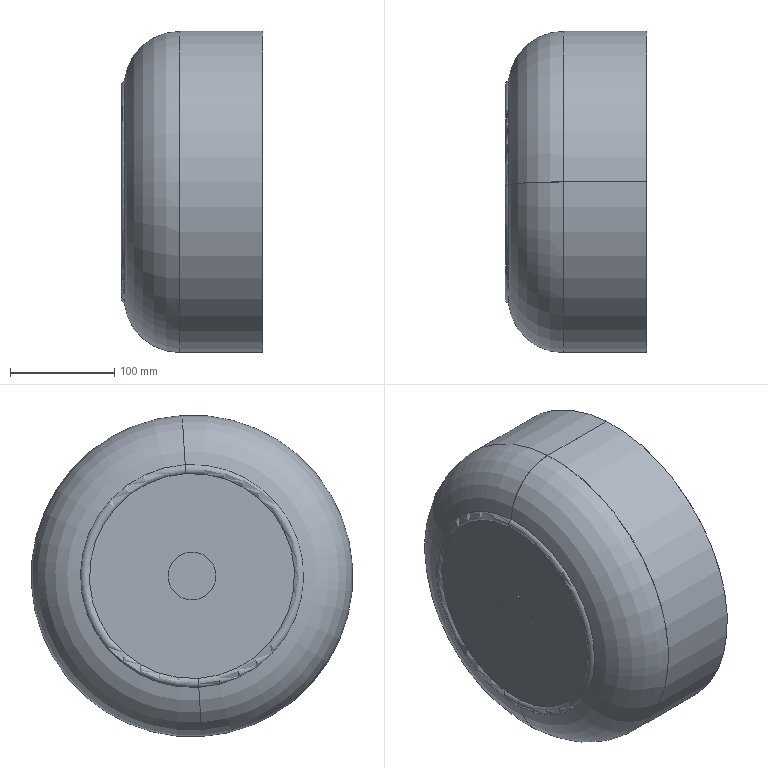Part | STEP file | Input 100 | 1 solid | 21 faces | box 136 x 309 x 309 mm | volume 181254 mm3 | cylinder 8 | torus 8 | plane 5 | commonest cylinder face diameters 44 x2 46 x2 307 x2 309 x2
STEP:
#1=CARTESIAN_POINT('',(0.,0.,0.));
#2=DIRECTION('',(0.,0.,1.));
#3=DIRECTION('',(1.,0.,0.));
#4=AXIS2_PLACEMENT_3D('',#1,#2,#3);
#5=CARTESIAN_POINT('',(3206.,663.657,-22.365));
#6=VERTEX_POINT('',#5);
#7=CARTESIAN_POINT('',(3207.,663.657,-22.365));
#8=VERTEX_POINT('',#7);
#9=CARTESIAN_POINT('',(3300.688,663.657,-22.365));
#10=DIRECTION('',(1.,0.,0.));
#11=VECTOR('',#10,1.);
#12=LINE('',#9,#11);
#13=CARTESIAN_POINT('',(3300.688,665.,-0.4063));
#14=DIRECTION('',(1.,0.,0.));
#15=DIRECTION('',(0.,-0.06105,-0.9981));
#16=AXIS2_PLACEMENT_3D('',#13,#14,#15);
#17=CYLINDRICAL_SURFACE('',#16,22.);
#18=CARTESIAN_POINT('',(6.283,0.));
#19=DIRECTION('',(0.,1.));
#20=VECTOR('',#19,1.);
#21=LINE('',#18,#20);
#22=(GEOMETRIC_REPRESENTATION_CONTEXT(2)PARAMETRIC_REPRESENTATION_CONTEXT()REPRESENTATION_CONTEXT('',''));
#23=DEFINITIONAL_REPRESENTATION('',(#21),#22);
#24=PCURVE('',#17,#23);
#25=CARTESIAN_POINT('',(3300.688,665.,-0.4063));
#26=DIRECTION('',(1.,0.,0.));
#27=DIRECTION('',(0.,-0.06105,-0.9981));
#28=AXIS2_PLACEMENT_3D('',#25,#26,#27);
#29=CYLINDRICAL_SURFACE('',#28,22.);
#30=CARTESIAN_POINT('',(0.,0.));
#31=DIRECTION('',(0.,1.));
#32=VECTOR('',#31,1.);
#33=LINE('',#30,#32);
#34=(GEOMETRIC_REPRESENTATION_CONTEXT(2)PARAMETRIC_REPRESENTATION_CONTEXT()REPRESENTATION_CONTEXT('',''));
#35=DEFINITIONAL_REPRESENTATION('',(#33),#34);
#36=PCURVE('',#29,#35);
#37=SURFACE_CURVE('',#12,(#24,#36),.PCURVE_S1.);
#38=EDGE_CURVE('',#6,#8,#37,.T.);
#39=ORIENTED_EDGE('',*,*,#38,.T.);
#40=CARTESIAN_POINT('',(3207.,666.343,21.553));
#41=VERTEX_POINT('',#40);
#42=CARTESIAN_POINT('',(3207.,665.,-0.4063));
#43=DIRECTION('',(1.,0.,0.));
#44=DIRECTION('',(0.,-0.06105,-0.9981));
#45=AXIS2_PLACEMENT_3D('',#42,#43,#44);
#46=CIRCLE('',#45,22.);
#47=CARTESIAN_POINT('',(0.,-93.688));
#48=DIRECTION('',(1.,0.));
#49=VECTOR('',#48,1.);
#50=LINE('',#47,#49);
#51=(GEOMETRIC_REPRESENTATION_CONTEXT(2)PARAMETRIC_REPRESENTATION_CONTEXT()REPRESENTATION_CONTEXT('',''));
#52=DEFINITIONAL_REPRESENTATION('',(#50),#51);
#53=PCURVE('',#17,#52);
#54=CARTESIAN_POINT('',(3207.,763.851,-6.452));
#55=DIRECTION('',(-1.,0.,0.));
#56=DIRECTION('',(0.,0.06105,0.9981));
#57=AXIS2_PLACEMENT_3D('',#54,#55,#56);
#58=PLANE('',#57);
#59=CARTESIAN_POINT('',(-22.,-99.036));
#60=CARTESIAN_POINT('',(-22.,-60.931));
#61=CARTESIAN_POINT('',(11.,-79.983));
#62=CARTESIAN_POINT('',(44.,-99.036));
#63=CARTESIAN_POINT('',(11.,-118.088));
#64=CARTESIAN_POINT('',(-22.,-137.141));
#65=CARTESIAN_POINT('',(-22.,-99.036));
#66=(BOUNDED_CURVE()B_SPLINE_CURVE(2,(#59,#60,#61,#62,#63,#64,#65),.UNSPECIFIED.,.T.,.F.)B_SPLINE_CURVE_WITH_KNOTS((1,2,2,2,2,1),(-2.094,0.,2.094,4.189,6.283,8.378),.UNSPECIFIED.)CURVE()GEOMETRIC_REPRESENTATION_ITEM()RATIONAL_B_SPLINE_CURVE((1.,0.5,1.,0.5,1.,0.5,1.))REPRESENTATION_ITEM(''));
#67=(GEOMETRIC_REPRESENTATION_CONTEXT(2)PARAMETRIC_REPRESENTATION_CONTEXT()REPRESENTATION_CONTEXT('',''));
#68=DEFINITIONAL_REPRESENTATION('',(#66),#67);
#69=PCURVE('',#58,#68);
#70=SURFACE_CURVE('',#46,(#53,#69),.PCURVE_S1.);
#71=EDGE_CURVE('',#41,#8,#70,.T.);
#72=ORIENTED_EDGE('',*,*,#71,.F.);
#73=CARTESIAN_POINT('',(3206.,666.343,21.553));
#74=VERTEX_POINT('',#73);
#75=CARTESIAN_POINT('',(3300.688,666.343,21.553));
#76=DIRECTION('',(1.,0.,0.));
#77=VECTOR('',#76,1.);
#78=LINE('',#75,#77);
#79=CARTESIAN_POINT('',(3.142,0.));
#80=DIRECTION('',(0.,1.));
#81=VECTOR('',#80,1.);
#82=LINE('',#79,#81);
#83=(GEOMETRIC_REPRESENTATION_CONTEXT(2)PARAMETRIC_REPRESENTATION_CONTEXT()REPRESENTATION_CONTEXT('',''));
#84=DEFINITIONAL_REPRESENTATION('',(#82),#83);
#85=PCURVE('',#17,#84);
#86=CARTESIAN_POINT('',(3.142,0.));
#87=DIRECTION('',(0.,1.));
#88=VECTOR('',#87,1.);
#89=LINE('',#86,#88);
#90=(GEOMETRIC_REPRESENTATION_CONTEXT(2)PARAMETRIC_REPRESENTATION_CONTEXT()REPRESENTATION_CONTEXT('',''));
#91=DEFINITIONAL_REPRESENTATION('',(#89),#90);
#92=PCURVE('',#29,#91);
#93=SURFACE_CURVE('',#78,(#85,#92),.PCURVE_S1.);
#94=EDGE_CURVE('',#74,#41,#93,.T.);
#95=ORIENTED_EDGE('',*,*,#94,.F.);
#96=CARTESIAN_POINT('',(3206.,665.,-0.4063));
#97=DIRECTION('',(1.,0.,0.));
#98=DIRECTION('',(0.,-0.06105,-0.9981));
#99=AXIS2_PLACEMENT_3D('',#96,#97,#98);
#100=CIRCLE('',#99,22.);
#101=CARTESIAN_POINT('',(0.,-94.688));
#102=DIRECTION('',(1.,0.));
#103=VECTOR('',#102,1.);
#104=LINE('',#101,#103);
#105=(GEOMETRIC_REPRESENTATION_CONTEXT(2)PARAMETRIC_REPRESENTATION_CONTEXT()REPRESENTATION_CONTEXT('',''));
#106=DEFINITIONAL_REPRESENTATION('',(#104),#105);
#107=PCURVE('',#17,#106);
#108=CARTESIAN_POINT('',(3206.,686.959,-1.749));
#109=DIRECTION('',(-1.,0.,0.));
#110=DIRECTION('',(0.,0.06105,0.9981));
#111=AXIS2_PLACEMENT_3D('',#108,#109,#110);
#112=PLANE('',#111);
#113=CARTESIAN_POINT('',(-22.,-22.));
#114=CARTESIAN_POINT('',(-22.,16.105));
#115=CARTESIAN_POINT('',(11.,-2.947));
#116=CARTESIAN_POINT('',(44.,-22.));
#117=CARTESIAN_POINT('',(11.,-41.053));
#118=CARTESIAN_POINT('',(-22.,-60.105));
#119=CARTESIAN_POINT('',(-22.,-22.));
#120=(BOUNDED_CURVE()B_SPLINE_CURVE(2,(#113,#114,#115,#116,#117,#118,#119),.UNSPECIFIED.,.T.,.F.)B_SPLINE_CURVE_WITH_KNOTS((1,2,2,2,2,1),(-2.094,0.,2.094,4.189,6.283,8.378),.UNSPECIFIED.)CURVE()GEOMETRIC_REPRESENTATION_ITEM()RATIONAL_B_SPLINE_CURVE((1.,0.5,1.,0.5,1.,0.5,1.))REPRESENTATION_ITEM(''));
#121=(GEOMETRIC_REPRESENTATION_CONTEXT(2)PARAMETRIC_REPRESENTATION_CONTEXT()REPRESENTATION_CONTEXT('',''));
#122=DEFINITIONAL_REPRESENTATION('',(#120),#121);
#123=PCURVE('',#112,#122);
#124=SURFACE_CURVE('',#100,(#107,#123),.PCURVE_S1.);
#125=EDGE_CURVE('',#74,#6,#124,.T.);
#126=ORIENTED_EDGE('',*,*,#125,.T.);
#127=EDGE_LOOP('',(#39,#72,#95,#126));
#128=FACE_BOUND('',#127,.F.);
#129=ADVANCED_FACE('',(#128),#17,.F.);
#130=CARTESIAN_POINT('',(3260.,655.629,-153.62));
#131=VERTEX_POINT('',#130);
#132=CARTESIAN_POINT('',(3340.,655.629,-153.62));
#133=VERTEX_POINT('',#132);
#134=CARTESIAN_POINT('',(3300.688,655.629,-153.62));
#135=DIRECTION('',(1.,0.,0.));
#136=VECTOR('',#135,1.);
#137=LINE('',#134,#136);
#138=CARTESIAN_POINT('',(3300.688,665.,-0.4063));
#139=DIRECTION('',(1.,0.,0.));
#140=DIRECTION('',(0.,-0.06105,-0.9981));
#141=AXIS2_PLACEMENT_3D('',#138,#139,#140);
#142=CYLINDRICAL_SURFACE('',#141,153.5);
#143=CARTESIAN_POINT('',(6.283,0.));
#144=DIRECTION('',(0.,1.));
#145=VECTOR('',#144,1.);
#146=LINE('',#143,#145);
#147=(GEOMETRIC_REPRESENTATION_CONTEXT(2)PARAMETRIC_REPRESENTATION_CONTEXT()REPRESENTATION_CONTEXT('',''));
#148=DEFINITIONAL_REPRESENTATION('',(#146),#147);
#149=PCURVE('',#142,#148);
#150=CARTESIAN_POINT('',(3300.688,665.,-0.4063));
#151=DIRECTION('',(1.,0.,0.));
#152=DIRECTION('',(0.,-0.06105,-0.9981));
#153=AXIS2_PLACEMENT_3D('',#150,#151,#152);
#154=CYLINDRICAL_SURFACE('',#153,153.5);
#155=CARTESIAN_POINT('',(0.,0.));
#156=DIRECTION('',(0.,1.));
#157=VECTOR('',#156,1.);
#158=LINE('',#155,#157);
#159=(GEOMETRIC_REPRESENTATION_CONTEXT(2)PARAMETRIC_REPRESENTATION_CONTEXT()REPRESENTATION_CONTEXT('',''));
#160=DEFINITIONAL_REPRESENTATION('',(#158),#159);
#161=PCURVE('',#154,#160);
#162=SURFACE_CURVE('',#137,(#149,#161),.PCURVE_S1.);
#163=EDGE_CURVE('',#131,#133,#162,.T.);
#164=ORIENTED_EDGE('',*,*,#163,.T.);
#165=CARTESIAN_POINT('',(3340.,674.371,152.807));
#166=VERTEX_POINT('',#165);
#167=CARTESIAN_POINT('',(3340.,665.,-0.4063));
#168=DIRECTION('',(1.,0.,0.));
#169=DIRECTION('',(0.,-0.06105,-0.9981));
#170=AXIS2_PLACEMENT_3D('',#167,#168,#169);
#171=CIRCLE('',#170,153.5);
#172=CARTESIAN_POINT('',(0.,39.312));
#173=DIRECTION('',(1.,0.));
#174=VECTOR('',#173,1.);
#175=LINE('',#172,#174);
#176=(GEOMETRIC_REPRESENTATION_CONTEXT(2)PARAMETRIC_REPRESENTATION_CONTEXT()REPRESENTATION_CONTEXT('',''));
#177=DEFINITIONAL_REPRESENTATION('',(#175),#176);
#178=PCURVE('',#142,#177);
#179=CARTESIAN_POINT('',(3340.,665.,-0.4063));
#180=DIRECTION('',(-1.,0.,0.));
#181=DIRECTION('',(0.,0.06105,0.9981));
#182=AXIS2_PLACEMENT_3D('',#179,#180,#181);
#183=PLANE('',#182);
#184=CARTESIAN_POINT('',(-153.5,0.));
#185=CARTESIAN_POINT('',(-153.5,265.87));
#186=CARTESIAN_POINT('',(76.75,132.935));
#187=CARTESIAN_POINT('',(307.,0.));
#188=CARTESIAN_POINT('',(76.75,-132.935));
#189=CARTESIAN_POINT('',(-153.5,-265.87));
#190=CARTESIAN_POINT('',(-153.5,0.));
#191=(BOUNDED_CURVE()B_SPLINE_CURVE(2,(#184,#185,#186,#187,#188,#189,#190),.UNSPECIFIED.,.T.,.F.)B_SPLINE_CURVE_WITH_KNOTS((1,2,2,2,2,1),(-2.094,0.,2.094,4.189,6.283,8.378),.UNSPECIFIED.)CURVE()GEOMETRIC_REPRESENTATION_ITEM()RATIONAL_B_SPLINE_CURVE((1.,0.5,1.,0.5,1.,0.5,1.))REPRESENTATION_ITEM(''));
#192=(GEOMETRIC_REPRESENTATION_CONTEXT(2)PARAMETRIC_REPRESENTATION_CONTEXT()REPRESENTATION_CONTEXT('',''));
#193=DEFINITIONAL_REPRESENTATION('',(#191),#192);
#194=PCURVE('',#183,#193);
#195=SURFACE_CURVE('',#171,(#178,#194),.PCURVE_S1.);
#196=EDGE_CURVE('',#166,#133,#195,.T.);
#197=ORIENTED_EDGE('',*,*,#196,.F.);
#198=CARTESIAN_POINT('',(3260.,674.371,152.807));
#199=VERTEX_POINT('',#198);
#200=CARTESIAN_POINT('',(3300.688,674.371,152.807));
#201=DIRECTION('',(1.,0.,0.));
#202=VECTOR('',#201,1.);
#203=LINE('',#200,#202);
#204=CARTESIAN_POINT('',(3.142,0.));
#205=DIRECTION('',(0.,1.));
#206=VECTOR('',#205,1.);
#207=LINE('',#204,#206);
#208=(GEOMETRIC_REPRESENTATION_CONTEXT(2)PARAMETRIC_REPRESENTATION_CONTEXT()REPRESENTATION_CONTEXT('',''));
#209=DEFINITIONAL_REPRESENTATION('',(#207),#208);
#210=PCURVE('',#142,#209);
#211=CARTESIAN_POINT('',(3.142,0.));
#212=DIRECTION('',(0.,1.));
#213=VECTOR('',#212,1.);
#214=LINE('',#211,#213);
#215=(GEOMETRIC_REPRESENTATION_CONTEXT(2)PARAMETRIC_REPRESENTATION_CONTEXT()REPRESENTATION_CONTEXT('',''));
#216=DEFINITIONAL_REPRESENTATION('',(#214),#215);
#217=PCURVE('',#154,#216);
#218=SURFACE_CURVE('',#203,(#210,#217),.PCURVE_S1.);
#219=EDGE_CURVE('',#199,#166,#218,.T.);
#220=ORIENTED_EDGE('',*,*,#219,.F.);
#221=CARTESIAN_POINT('',(3260.,665.,-0.4063));
#222=DIRECTION('',(1.,0.,0.));
#223=DIRECTION('',(0.,-0.06105,-0.9981));
#224=AXIS2_PLACEMENT_3D('',#221,#222,#223);
#225=CIRCLE('',#224,153.5);
#226=CARTESIAN_POINT('',(0.,-40.688));
#227=DIRECTION('',(1.,0.));
#228=VECTOR('',#227,1.);
#229=LINE('',#226,#228);
#230=(GEOMETRIC_REPRESENTATION_CONTEXT(2)PARAMETRIC_REPRESENTATION_CONTEXT()REPRESENTATION_CONTEXT('',''));
#231=DEFINITIONAL_REPRESENTATION('',(#229),#230);
#232=PCURVE('',#142,#231);
#233=CARTESIAN_POINT('',(3260.,665.,-0.4063));
#234=DIRECTION('',(1.,0.,0.));
#235=DIRECTION('',(0.,-0.06105,-0.9981));
#236=AXIS2_PLACEMENT_3D('',#233,#234,#235);
#237=TOROIDAL_SURFACE('',#236,101.248,52.252);
#238=CARTESIAN_POINT('',(0.,6.283));
#239=DIRECTION('',(1.,0.));
#240=VECTOR('',#239,1.);
#241=LINE('',#238,#240);
#242=(GEOMETRIC_REPRESENTATION_CONTEXT(2)PARAMETRIC_REPRESENTATION_CONTEXT()REPRESENTATION_CONTEXT('',''));
#243=DEFINITIONAL_REPRESENTATION('',(#241),#242);
#244=PCURVE('',#237,#243);
#245=SURFACE_CURVE('',#225,(#232,#244),.PCURVE_S1.);
#246=EDGE_CURVE('',#199,#131,#245,.T.);
#247=ORIENTED_EDGE('',*,*,#246,.T.);
#248=EDGE_LOOP('',(#164,#197,#220,#247));
#249=FACE_BOUND('',#248,.F.);
#250=ADVANCED_FACE('',(#249),#142,.F.);
#251=CARTESIAN_POINT('',(3207.,658.954,-99.257));
#252=VERTEX_POINT('',#251);
#253=CARTESIAN_POINT('',(3208.,658.506,-106.581));
#254=VERTEX_POINT('',#253);
#255=CARTESIAN_POINT('',(3209.,658.743,-102.715));
#256=DIRECTION('',(0.,-0.9981,0.06105));
#257=DIRECTION('',(0.,-0.06105,-0.9981));
#258=AXIS2_PLACEMENT_3D('',#255,#256,#257);
#259=CIRCLE('',#258,4.);
#260=CARTESIAN_POINT('',(3209.,665.,-0.4063));
#261=DIRECTION('',(1.,0.,0.));
#262=DIRECTION('',(0.,-0.06105,-0.9981));
#263=AXIS2_PLACEMENT_3D('',#260,#261,#262);
#264=TOROIDAL_SURFACE('',#263,102.5,4.);
#265=CARTESIAN_POINT('',(6.283,0.));
#266=DIRECTION('',(0.,1.));
#267=VECTOR('',#266,1.);
#268=LINE('',#265,#267);
#269=(GEOMETRIC_REPRESENTATION_CONTEXT(2)PARAMETRIC_REPRESENTATION_CONTEXT()REPRESENTATION_CONTEXT('',''));
#270=DEFINITIONAL_REPRESENTATION('',(#268),#269);
#271=PCURVE('',#264,#270);
#272=CARTESIAN_POINT('',(3209.,665.,-0.4063));
#273=DIRECTION('',(1.,0.,0.));
#274=DIRECTION('',(0.,-0.06105,-0.9981));
#275=AXIS2_PLACEMENT_3D('',#272,#273,#274);
#276=TOROIDAL_SURFACE('',#275,102.5,4.);
#277=CARTESIAN_POINT('',(0.,0.));
#278=DIRECTION('',(0.,1.));
#279=VECTOR('',#278,1.);
#280=LINE('',#277,#279);
#281=(GEOMETRIC_REPRESENTATION_CONTEXT(2)PARAMETRIC_REPRESENTATION_CONTEXT()REPRESENTATION_CONTEXT('',''));
#282=DEFINITIONAL_REPRESENTATION('',(#280),#281);
#283=PCURVE('',#276,#282);
#284=SURFACE_CURVE('',#259,(#271,#283),.PCURVE_S1.);
#285=EDGE_CURVE('',#252,#254,#284,.T.);
#286=ORIENTED_EDGE('',*,*,#285,.T.);
#287=CARTESIAN_POINT('',(3208.,671.494,105.768));
#288=VERTEX_POINT('',#287);
#289=CARTESIAN_POINT('',(3208.,665.,-0.4063));
#290=DIRECTION('',(1.,0.,0.));
#291=DIRECTION('',(0.,-0.06105,-0.9981));
#292=AXIS2_PLACEMENT_3D('',#289,#290,#291);
#293=CIRCLE('',#292,106.373);
#294=CARTESIAN_POINT('',(0.,6.031));
#295=DIRECTION('',(1.,0.));
#296=VECTOR('',#295,1.);
#297=LINE('',#294,#296);
#298=(GEOMETRIC_REPRESENTATION_CONTEXT(2)PARAMETRIC_REPRESENTATION_CONTEXT()REPRESENTATION_CONTEXT('',''));
#299=DEFINITIONAL_REPRESENTATION('',(#297),#298);
#300=PCURVE('',#264,#299);
#301=CARTESIAN_POINT('',(0.,4.811));
#302=DIRECTION('',(1.,0.));
#303=VECTOR('',#302,1.);
#304=LINE('',#301,#303);
#305=(GEOMETRIC_REPRESENTATION_CONTEXT(2)PARAMETRIC_REPRESENTATION_CONTEXT()REPRESENTATION_CONTEXT('',''));
#306=DEFINITIONAL_REPRESENTATION('',(#304),#305);
#307=PCURVE('',#237,#306);
#308=SURFACE_CURVE('',#293,(#300,#307),.PCURVE_S1.);
#309=EDGE_CURVE('',#288,#254,#308,.T.);
#310=ORIENTED_EDGE('',*,*,#309,.F.);
#311=CARTESIAN_POINT('',(3207.,671.046,98.445));
#312=VERTEX_POINT('',#311);
#313=CARTESIAN_POINT('',(3209.,671.257,101.902));
#314=DIRECTION('',(0.,0.9981,-0.06105));
#315=DIRECTION('',(0.,0.06105,0.9981));
#316=AXIS2_PLACEMENT_3D('',#313,#314,#315);
#317=CIRCLE('',#316,4.);
#318=CARTESIAN_POINT('',(3.142,0.));
#319=DIRECTION('',(0.,1.));
#320=VECTOR('',#319,1.);
#321=LINE('',#318,#320);
#322=(GEOMETRIC_REPRESENTATION_CONTEXT(2)PARAMETRIC_REPRESENTATION_CONTEXT()REPRESENTATION_CONTEXT('',''));
#323=DEFINITIONAL_REPRESENTATION('',(#321),#322);
#324=PCURVE('',#264,#323);
#325=CARTESIAN_POINT('',(3.142,0.));
#326=DIRECTION('',(0.,1.));
#327=VECTOR('',#326,1.);
#328=LINE('',#325,#327);
#329=(GEOMETRIC_REPRESENTATION_CONTEXT(2)PARAMETRIC_REPRESENTATION_CONTEXT()REPRESENTATION_CONTEXT('',''));
#330=DEFINITIONAL_REPRESENTATION('',(#328),#329);
#331=PCURVE('',#276,#330);
#332=SURFACE_CURVE('',#317,(#324,#331),.PCURVE_S1.);
#333=EDGE_CURVE('',#312,#288,#332,.T.);
#334=ORIENTED_EDGE('',*,*,#333,.F.);
#335=CARTESIAN_POINT('',(3207.,665.,-0.4063));
#336=DIRECTION('',(1.,0.,0.));
#337=DIRECTION('',(0.,-0.06105,-0.9981));
#338=AXIS2_PLACEMENT_3D('',#335,#336,#337);
#339=CIRCLE('',#338,99.036);
#340=CARTESIAN_POINT('',(0.,3.665));
#341=DIRECTION('',(1.,0.));
#342=VECTOR('',#341,1.);
#343=LINE('',#340,#342);
#344=(GEOMETRIC_REPRESENTATION_CONTEXT(2)PARAMETRIC_REPRESENTATION_CONTEXT()REPRESENTATION_CONTEXT('',''));
#345=DEFINITIONAL_REPRESENTATION('',(#343),#344);
#346=PCURVE('',#264,#345);
#347=CARTESIAN_POINT('',(-99.036,-99.036));
#348=CARTESIAN_POINT('',(-99.036,72.499));
#349=CARTESIAN_POINT('',(49.518,-13.268));
#350=CARTESIAN_POINT('',(198.072,-99.036));
#351=CARTESIAN_POINT('',(49.518,-184.804));
#352=CARTESIAN_POINT('',(-99.036,-270.571));
#353=CARTESIAN_POINT('',(-99.036,-99.036));
#354=(BOUNDED_CURVE()B_SPLINE_CURVE(2,(#347,#348,#349,#350,#351,#352,#353),.UNSPECIFIED.,.T.,.F.)B_SPLINE_CURVE_WITH_KNOTS((1,2,2,2,2,1),(-2.094,0.,2.094,4.189,6.283,8.378),.UNSPECIFIED.)CURVE()GEOMETRIC_REPRESENTATION_ITEM()RATIONAL_B_SPLINE_CURVE((1.,0.5,1.,0.5,1.,0.5,1.))REPRESENTATION_ITEM(''));
#355=(GEOMETRIC_REPRESENTATION_CONTEXT(2)PARAMETRIC_REPRESENTATION_CONTEXT()REPRESENTATION_CONTEXT('',''));
#356=DEFINITIONAL_REPRESENTATION('',(#354),#355);
#357=PCURVE('',#58,#356);
#358=SURFACE_CURVE('',#339,(#346,#357),.PCURVE_S1.);
#359=EDGE_CURVE('',#312,#252,#358,.T.);
#360=ORIENTED_EDGE('',*,*,#359,.T.);
#361=EDGE_LOOP('',(#286,#310,#334,#360));
#362=FACE_BOUND('',#361,.F.);
#363=ADVANCED_FACE('',(#362),#264,.F.);
#364=CARTESIAN_POINT('',(3260.,658.819,-101.466));
#365=DIRECTION('',(0.,-0.9981,0.06105));
#366=DIRECTION('',(0.,-0.06105,-0.9981));
#367=AXIS2_PLACEMENT_3D('',#364,#365,#366);
#368=CIRCLE('',#367,52.252);
#369=CARTESIAN_POINT('',(6.283,0.));
#370=DIRECTION('',(0.,1.));
#371=VECTOR('',#370,1.);
#372=LINE('',#369,#371);
#373=(GEOMETRIC_REPRESENTATION_CONTEXT(2)PARAMETRIC_REPRESENTATION_CONTEXT()REPRESENTATION_CONTEXT('',''));
#374=DEFINITIONAL_REPRESENTATION('',(#372),#373);
#375=PCURVE('',#237,#374);
#376=CARTESIAN_POINT('',(3260.,665.,-0.4063));
#377=DIRECTION('',(1.,0.,0.));
#378=DIRECTION('',(0.,-0.06105,-0.9981));
#379=AXIS2_PLACEMENT_3D('',#376,#377,#378);
#380=TOROIDAL_SURFACE('',#379,101.248,52.252);
#381=CARTESIAN_POINT('',(0.,0.));
#382=DIRECTION('',(0.,1.));
#383=VECTOR('',#382,1.);
#384=LINE('',#381,#383);
#385=(GEOMETRIC_REPRESENTATION_CONTEXT(2)PARAMETRIC_REPRESENTATION_CONTEXT()REPRESENTATION_CONTEXT('',''));
#386=DEFINITIONAL_REPRESENTATION('',(#384),#385);
#387=PCURVE('',#380,#386);
#388=SURFACE_CURVE('',#368,(#375,#387),.PCURVE_S1.);
#389=EDGE_CURVE('',#254,#131,#388,.T.);
#390=ORIENTED_EDGE('',*,*,#389,.T.);
#391=ORIENTED_EDGE('',*,*,#246,.F.);
#392=CARTESIAN_POINT('',(3260.,671.181,100.653));
#393=DIRECTION('',(0.,0.9981,-0.06105));
#394=DIRECTION('',(0.,0.06105,0.9981));
#395=AXIS2_PLACEMENT_3D('',#392,#393,#394);
#396=CIRCLE('',#395,52.252);
#397=CARTESIAN_POINT('',(3.142,0.));
#398=DIRECTION('',(0.,1.));
#399=VECTOR('',#398,1.);
#400=LINE('',#397,#399);
#401=(GEOMETRIC_REPRESENTATION_CONTEXT(2)PARAMETRIC_REPRESENTATION_CONTEXT()REPRESENTATION_CONTEXT('',''));
#402=DEFINITIONAL_REPRESENTATION('',(#400),#401);
#403=PCURVE('',#237,#402);
#404=CARTESIAN_POINT('',(3.142,0.));
#405=DIRECTION('',(0.,1.));
#406=VECTOR('',#405,1.);
#407=LINE('',#404,#406);
#408=(GEOMETRIC_REPRESENTATION_CONTEXT(2)PARAMETRIC_REPRESENTATION_CONTEXT()REPRESENTATION_CONTEXT('',''));
#409=DEFINITIONAL_REPRESENTATION('',(#407),#408);
#410=PCURVE('',#380,#409);
#411=SURFACE_CURVE('',#396,(#403,#410),.PCURVE_S1.);
#412=EDGE_CURVE('',#288,#199,#411,.T.);
#413=ORIENTED_EDGE('',*,*,#412,.F.);
#414=ORIENTED_EDGE('',*,*,#309,.T.);
#415=EDGE_LOOP('',(#390,#391,#413,#414));
#416=FACE_BOUND('',#415,.F.);
#417=ADVANCED_FACE('',(#416),#237,.F.);
#418=CARTESIAN_POINT('',(3205.,663.596,-23.363));
#419=VERTEX_POINT('',#418);
#420=CARTESIAN_POINT('',(3205.,666.404,22.551));
#421=VERTEX_POINT('',#420);
#422=CARTESIAN_POINT('',(3205.,665.,-0.4063));
#423=DIRECTION('',(1.,0.,0.));
#424=DIRECTION('',(0.,0.06105,0.9981));
#425=AXIS2_PLACEMENT_3D('',#422,#423,#424);
#426=CIRCLE('',#425,23.);
#427=CARTESIAN_POINT('',(3300.688,665.,-0.4063));
#428=DIRECTION('',(1.,0.,0.));
#429=DIRECTION('',(0.,-0.06105,-0.9981));
#430=AXIS2_PLACEMENT_3D('',#427,#428,#429);
#431=CYLINDRICAL_SURFACE('',#430,23.);
#432=CARTESIAN_POINT('',(-3.142,-95.688));
#433=DIRECTION('',(1.,0.));
#434=VECTOR('',#433,1.);
#435=LINE('',#432,#434);
#436=(GEOMETRIC_REPRESENTATION_CONTEXT(2)PARAMETRIC_REPRESENTATION_CONTEXT()REPRESENTATION_CONTEXT('',''));
#437=DEFINITIONAL_REPRESENTATION('',(#435),#436);
#438=PCURVE('',#431,#437);
#439=CARTESIAN_POINT('',(3205.,686.959,-1.749));
#440=DIRECTION('',(-1.,0.,0.));
#441=DIRECTION('',(0.,0.06105,0.9981));
#442=AXIS2_PLACEMENT_3D('',#439,#440,#441);
#443=PLANE('',#442);
#444=CARTESIAN_POINT('',(23.,-22.));
#445=CARTESIAN_POINT('',(23.,-61.837));
#446=CARTESIAN_POINT('',(-11.5,-41.919));
#447=CARTESIAN_POINT('',(-46.,-22.));
#448=CARTESIAN_POINT('',(-11.5,-2.081));
#449=CARTESIAN_POINT('',(23.,17.837));
#450=CARTESIAN_POINT('',(23.,-22.));
#451=(BOUNDED_CURVE()B_SPLINE_CURVE(2,(#444,#445,#446,#447,#448,#449,#450),.UNSPECIFIED.,.T.,.F.)B_SPLINE_CURVE_WITH_KNOTS((1,2,2,2,2,1),(-2.094,0.,2.094,4.189,6.283,8.378),.UNSPECIFIED.)CURVE()GEOMETRIC_REPRESENTATION_ITEM()RATIONAL_B_SPLINE_CURVE((1.,0.5,1.,0.5,1.,0.5,1.))REPRESENTATION_ITEM(''));
#452=(GEOMETRIC_REPRESENTATION_CONTEXT(2)PARAMETRIC_REPRESENTATION_CONTEXT()REPRESENTATION_CONTEXT('',''));
#453=DEFINITIONAL_REPRESENTATION('',(#451),#452);
#454=PCURVE('',#443,#453);
#455=SURFACE_CURVE('',#426,(#438,#454),.PCURVE_S1.);
#456=EDGE_CURVE('',#419,#421,#455,.T.);
#457=ORIENTED_EDGE('',*,*,#456,.T.);
#458=CARTESIAN_POINT('',(3206.,666.404,22.551));
#459=VERTEX_POINT('',#458);
#460=CARTESIAN_POINT('',(3300.688,666.404,22.551));
#461=DIRECTION('',(1.,0.,0.));
#462=VECTOR('',#461,1.);
#463=LINE('',#460,#462);
#464=CARTESIAN_POINT('',(3.142,0.));
#465=DIRECTION('',(0.,1.));
#466=VECTOR('',#465,1.);
#467=LINE('',#464,#466);
#468=(GEOMETRIC_REPRESENTATION_CONTEXT(2)PARAMETRIC_REPRESENTATION_CONTEXT()REPRESENTATION_CONTEXT('',''));
#469=DEFINITIONAL_REPRESENTATION('',(#467),#468);
#470=PCURVE('',#431,#469);
#471=CARTESIAN_POINT('',(3300.688,665.,-0.4063));
#472=DIRECTION('',(1.,0.,0.));
#473=DIRECTION('',(0.,-0.06105,-0.9981));
#474=AXIS2_PLACEMENT_3D('',#471,#472,#473);
#475=CYLINDRICAL_SURFACE('',#474,23.);
#476=CARTESIAN_POINT('',(3.142,0.));
#477=DIRECTION('',(0.,1.));
#478=VECTOR('',#477,1.);
#479=LINE('',#476,#478);
#480=(GEOMETRIC_REPRESENTATION_CONTEXT(2)PARAMETRIC_REPRESENTATION_CONTEXT()REPRESENTATION_CONTEXT('',''));
#481=DEFINITIONAL_REPRESENTATION('',(#479),#480);
#482=PCURVE('',#475,#481);
#483=SURFACE_CURVE('',#463,(#470,#482),.PCURVE_S1.);
#484=EDGE_CURVE('',#421,#459,#483,.T.);
#485=ORIENTED_EDGE('',*,*,#484,.T.);
#486=CARTESIAN_POINT('',(3206.,663.596,-23.363));
#487=VERTEX_POINT('',#486);
#488=CARTESIAN_POINT('',(3206.,665.,-0.4063));
#489=DIRECTION('',(1.,0.,0.));
#490=DIRECTION('',(0.,0.06105,0.9981));
#491=AXIS2_PLACEMENT_3D('',#488,#489,#490);
#492=CIRCLE('',#491,23.);
#493=CARTESIAN_POINT('',(-3.142,-94.688));
#494=DIRECTION('',(1.,0.));
#495=VECTOR('',#494,1.);
#496=LINE('',#493,#495);
#497=(GEOMETRIC_REPRESENTATION_CONTEXT(2)PARAMETRIC_REPRESENTATION_CONTEXT()REPRESENTATION_CONTEXT('',''));
#498=DEFINITIONAL_REPRESENTATION('',(#496),#497);
#499=PCURVE('',#431,#498);
#500=CARTESIAN_POINT('',(3206.,763.851,-6.452));
#501=DIRECTION('',(-1.,0.,0.));
#502=DIRECTION('',(0.,0.06105,0.9981));
#503=AXIS2_PLACEMENT_3D('',#500,#501,#502);
#504=PLANE('',#503);
#505=CARTESIAN_POINT('',(23.,-99.036));
#506=CARTESIAN_POINT('',(23.,-138.873));
#507=CARTESIAN_POINT('',(-11.5,-118.954));
#508=CARTESIAN_POINT('',(-46.,-99.036));
#509=CARTESIAN_POINT('',(-11.5,-79.117));
#510=CARTESIAN_POINT('',(23.,-59.199));
#511=CARTESIAN_POINT('',(23.,-99.036));
#512=(BOUNDED_CURVE()B_SPLINE_CURVE(2,(#505,#506,#507,#508,#509,#510,#511),.UNSPECIFIED.,.T.,.F.)B_SPLINE_CURVE_WITH_KNOTS((1,2,2,2,2,1),(-2.094,0.,2.094,4.189,6.283,8.378),.UNSPECIFIED.)CURVE()GEOMETRIC_REPRESENTATION_ITEM()RATIONAL_B_SPLINE_CURVE((1.,0.5,1.,0.5,1.,0.5,1.))REPRESENTATION_ITEM(''));
#513=(GEOMETRIC_REPRESENTATION_CONTEXT(2)PARAMETRIC_REPRESENTATION_CONTEXT()REPRESENTATION_CONTEXT('',''));
#514=DEFINITIONAL_REPRESENTATION('',(#512),#513);
#515=PCURVE('',#504,#514);
#516=SURFACE_CURVE('',#492,(#499,#515),.PCURVE_S1.);
#517=EDGE_CURVE('',#487,#459,#516,.T.);
#518=ORIENTED_EDGE('',*,*,#517,.F.);
#519=CARTESIAN_POINT('',(3300.688,663.596,-23.363));
#520=DIRECTION('',(1.,0.,0.));
#521=VECTOR('',#520,1.);
#522=LINE('',#519,#521);
#523=CARTESIAN_POINT('',(0.,0.));
#524=DIRECTION('',(0.,1.));
#525=VECTOR('',#524,1.);
#526=LINE('',#523,#525);
#527=(GEOMETRIC_REPRESENTATION_CONTEXT(2)PARAMETRIC_REPRESENTATION_CONTEXT()REPRESENTATION_CONTEXT('',''));
#528=DEFINITIONAL_REPRESENTATION('',(#526),#527);
#529=PCURVE('',#431,#528);
#530=CARTESIAN_POINT('',(6.283,0.));
#531=DIRECTION('',(0.,1.));
#532=VECTOR('',#531,1.);
#533=LINE('',#530,#532);
#534=(GEOMETRIC_REPRESENTATION_CONTEXT(2)PARAMETRIC_REPRESENTATION_CONTEXT()REPRESENTATION_CONTEXT('',''));
#535=DEFINITIONAL_REPRESENTATION('',(#533),#534);
#536=PCURVE('',#475,#535);
#537=SURFACE_CURVE('',#522,(#529,#536),.PCURVE_S1.);
#538=EDGE_CURVE('',#419,#487,#537,.T.);
#539=ORIENTED_EDGE('',*,*,#538,.F.);
#540=EDGE_LOOP('',(#457,#485,#518,#539));
#541=FACE_BOUND('',#540,.T.);
#542=ADVANCED_FACE('',(#541),#431,.T.);
#543=CARTESIAN_POINT('',(3260.,655.568,-154.618));
#544=VERTEX_POINT('',#543);
#545=CARTESIAN_POINT('',(3260.,674.432,153.806));
#546=VERTEX_POINT('',#545);
#547=CARTESIAN_POINT('',(3260.,665.,-0.4063));
#548=DIRECTION('',(1.,0.,0.));
#549=DIRECTION('',(0.,-0.06105,-0.9981));
#550=AXIS2_PLACEMENT_3D('',#547,#548,#549);
#551=CIRCLE('',#550,154.5);
#552=CARTESIAN_POINT('',(3300.688,665.,-0.4063));
#553=DIRECTION('',(1.,0.,0.));
#554=DIRECTION('',(0.,-0.06105,-0.9981));
#555=AXIS2_PLACEMENT_3D('',#552,#553,#554);
#556=CYLINDRICAL_SURFACE('',#555,154.5);
#557=CARTESIAN_POINT('',(0.,-40.688));
#558=DIRECTION('',(1.,0.));
#559=VECTOR('',#558,1.);
#560=LINE('',#557,#559);
#561=(GEOMETRIC_REPRESENTATION_CONTEXT(2)PARAMETRIC_REPRESENTATION_CONTEXT()REPRESENTATION_CONTEXT('',''));
#562=DEFINITIONAL_REPRESENTATION('',(#560),#561);
#563=PCURVE('',#556,#562);
#564=CARTESIAN_POINT('',(3260.,665.,-0.4063));
#565=DIRECTION('',(1.,0.,0.));
#566=DIRECTION('',(0.,-0.06105,-0.9981));
#567=AXIS2_PLACEMENT_3D('',#564,#565,#566);
#568=TOROIDAL_SURFACE('',#567,101.248,53.252);
#569=CARTESIAN_POINT('',(0.,6.283));
#570=DIRECTION('',(1.,0.));
#571=VECTOR('',#570,1.);
#572=LINE('',#569,#571);
#573=(GEOMETRIC_REPRESENTATION_CONTEXT(2)PARAMETRIC_REPRESENTATION_CONTEXT()REPRESENTATION_CONTEXT('',''));
#574=DEFINITIONAL_REPRESENTATION('',(#572),#573);
#575=PCURVE('',#568,#574);
#576=SURFACE_CURVE('',#551,(#563,#575),.PCURVE_S1.);
#577=EDGE_CURVE('',#544,#546,#576,.T.);
#578=ORIENTED_EDGE('',*,*,#577,.T.);
#579=CARTESIAN_POINT('',(3340.,674.432,153.806));
#580=VERTEX_POINT('',#579);
#581=CARTESIAN_POINT('',(3300.688,674.432,153.806));
#582=DIRECTION('',(1.,0.,0.));
#583=VECTOR('',#582,1.);
#584=LINE('',#581,#583);
#585=CARTESIAN_POINT('',(3.142,0.));
#586=DIRECTION('',(0.,1.));
#587=VECTOR('',#586,1.);
#588=LINE('',#585,#587);
#589=(GEOMETRIC_REPRESENTATION_CONTEXT(2)PARAMETRIC_REPRESENTATION_CONTEXT()REPRESENTATION_CONTEXT('',''));
#590=DEFINITIONAL_REPRESENTATION('',(#588),#589);
#591=PCURVE('',#556,#590);
#592=CARTESIAN_POINT('',(3300.688,665.,-0.4063));
#593=DIRECTION('',(1.,0.,0.));
#594=DIRECTION('',(0.,-0.06105,-0.9981));
#595=AXIS2_PLACEMENT_3D('',#592,#593,#594);
#596=CYLINDRICAL_SURFACE('',#595,154.5);
#597=CARTESIAN_POINT('',(3.142,0.));
#598=DIRECTION('',(0.,1.));
#599=VECTOR('',#598,1.);
#600=LINE('',#597,#599);
#601=(GEOMETRIC_REPRESENTATION_CONTEXT(2)PARAMETRIC_REPRESENTATION_CONTEXT()REPRESENTATION_CONTEXT('',''));
#602=DEFINITIONAL_REPRESENTATION('',(#600),#601);
#603=PCURVE('',#596,#602);
#604=SURFACE_CURVE('',#584,(#591,#603),.PCURVE_S1.);
#605=EDGE_CURVE('',#546,#580,#604,.T.);
#606=ORIENTED_EDGE('',*,*,#605,.T.);
#607=CARTESIAN_POINT('',(3340.,655.568,-154.618));
#608=VERTEX_POINT('',#607);
#609=CARTESIAN_POINT('',(3340.,665.,-0.4063));
#610=DIRECTION('',(1.,0.,0.));
#611=DIRECTION('',(0.,-0.06105,-0.9981));
#612=AXIS2_PLACEMENT_3D('',#609,#610,#611);
#613=CIRCLE('',#612,154.5);
#614=CARTESIAN_POINT('',(0.,39.312));
#615=DIRECTION('',(1.,0.));
#616=VECTOR('',#615,1.);
#617=LINE('',#614,#616);
#618=(GEOMETRIC_REPRESENTATION_CONTEXT(2)PARAMETRIC_REPRESENTATION_CONTEXT()REPRESENTATION_CONTEXT('',''));
#619=DEFINITIONAL_REPRESENTATION('',(#617),#618);
#620=PCURVE('',#556,#619);
#621=CARTESIAN_POINT('',(-154.5,0.));
#622=CARTESIAN_POINT('',(-154.5,267.602));
#623=CARTESIAN_POINT('',(77.25,133.801));
#624=CARTESIAN_POINT('',(309.,0.));
#625=CARTESIAN_POINT('',(77.25,-133.801));
#626=CARTESIAN_POINT('',(-154.5,-267.602));
#627=CARTESIAN_POINT('',(-154.5,0.));
#628=(BOUNDED_CURVE()B_SPLINE_CURVE(2,(#621,#622,#623,#624,#625,#626,#627),.UNSPECIFIED.,.T.,.F.)B_SPLINE_CURVE_WITH_KNOTS((1,2,2,2,2,1),(-2.094,0.,2.094,4.189,6.283,8.378),.UNSPECIFIED.)CURVE()GEOMETRIC_REPRESENTATION_ITEM()RATIONAL_B_SPLINE_CURVE((1.,0.5,1.,0.5,1.,0.5,1.))REPRESENTATION_ITEM(''));
#629=(GEOMETRIC_REPRESENTATION_CONTEXT(2)PARAMETRIC_REPRESENTATION_CONTEXT()REPRESENTATION_CONTEXT('',''));
#630=DEFINITIONAL_REPRESENTATION('',(#628),#629);
#631=PCURVE('',#183,#630);
#632=SURFACE_CURVE('',#613,(#620,#631),.PCURVE_S1.);
#633=EDGE_CURVE('',#608,#580,#632,.T.);
#634=ORIENTED_EDGE('',*,*,#633,.F.);
#635=CARTESIAN_POINT('',(3300.688,655.568,-154.618));
#636=DIRECTION('',(1.,0.,0.));
#637=VECTOR('',#636,1.);
#638=LINE('',#635,#637);
#639=CARTESIAN_POINT('',(0.,0.));
#640=DIRECTION('',(0.,1.));
#641=VECTOR('',#640,1.);
#642=LINE('',#639,#641);
#643=(GEOMETRIC_REPRESENTATION_CONTEXT(2)PARAMETRIC_REPRESENTATION_CONTEXT()REPRESENTATION_CONTEXT('',''));
#644=DEFINITIONAL_REPRESENTATION('',(#642),#643);
#645=PCURVE('',#556,#644);
#646=CARTESIAN_POINT('',(6.283,0.));
#647=DIRECTION('',(0.,1.));
#648=VECTOR('',#647,1.);
#649=LINE('',#646,#648);
#650=(GEOMETRIC_REPRESENTATION_CONTEXT(2)PARAMETRIC_REPRESENTATION_CONTEXT()REPRESENTATION_CONTEXT('',''));
#651=DEFINITIONAL_REPRESENTATION('',(#649),#650);
#652=PCURVE('',#596,#651);
#653=SURFACE_CURVE('',#638,(#645,#652),.PCURVE_S1.);
#654=EDGE_CURVE('',#544,#608,#653,.T.);
#655=ORIENTED_EDGE('',*,*,#654,.F.);
#656=EDGE_LOOP('',(#578,#606,#634,#655));
#657=FACE_BOUND('',#656,.T.);
#658=ADVANCED_FACE('',(#657),#556,.T.);
#659=CARTESIAN_POINT('',(3206.,658.987,-98.723));
#660=VERTEX_POINT('',#659);
#661=CARTESIAN_POINT('',(3206.,671.013,97.91));
#662=VERTEX_POINT('',#661);
#663=CARTESIAN_POINT('',(3206.,665.,-0.4063));
#664=DIRECTION('',(1.,0.,0.));
#665=DIRECTION('',(0.,-0.06105,-0.9981));
#666=AXIS2_PLACEMENT_3D('',#663,#664,#665);
#667=CIRCLE('',#666,98.5);
#668=CARTESIAN_POINT('',(3209.,665.,-0.4063));
#669=DIRECTION('',(1.,0.,0.));
#670=DIRECTION('',(0.,-0.06105,-0.9981));
#671=AXIS2_PLACEMENT_3D('',#668,#669,#670);
#672=TOROIDAL_SURFACE('',#671,102.5,5.);
#673=CARTESIAN_POINT('',(0.,3.785));
#674=DIRECTION('',(1.,0.));
#675=VECTOR('',#674,1.);
#676=LINE('',#673,#675);
#677=(GEOMETRIC_REPRESENTATION_CONTEXT(2)PARAMETRIC_REPRESENTATION_CONTEXT()REPRESENTATION_CONTEXT('',''));
#678=DEFINITIONAL_REPRESENTATION('',(#676),#677);
#679=PCURVE('',#672,#678);
#680=CARTESIAN_POINT('',(-98.5,-99.036));
#681=CARTESIAN_POINT('',(-98.5,71.571));
#682=CARTESIAN_POINT('',(49.25,-13.732));
#683=CARTESIAN_POINT('',(197.,-99.036));
#684=CARTESIAN_POINT('',(49.25,-184.339));
#685=CARTESIAN_POINT('',(-98.5,-269.643));
#686=CARTESIAN_POINT('',(-98.5,-99.036));
#687=(BOUNDED_CURVE()B_SPLINE_CURVE(2,(#680,#681,#682,#683,#684,#685,#686),.UNSPECIFIED.,.T.,.F.)B_SPLINE_CURVE_WITH_KNOTS((1,2,2,2,2,1),(-2.094,0.,2.094,4.189,6.283,8.378),.UNSPECIFIED.)CURVE()GEOMETRIC_REPRESENTATION_ITEM()RATIONAL_B_SPLINE_CURVE((1.,0.5,1.,0.5,1.,0.5,1.))REPRESENTATION_ITEM(''));
#688=(GEOMETRIC_REPRESENTATION_CONTEXT(2)PARAMETRIC_REPRESENTATION_CONTEXT()REPRESENTATION_CONTEXT('',''));
#689=DEFINITIONAL_REPRESENTATION('',(#687),#688);
#690=PCURVE('',#504,#689);
#691=SURFACE_CURVE('',#667,(#679,#690),.PCURVE_S1.);
#692=EDGE_CURVE('',#660,#662,#691,.T.);
#693=ORIENTED_EDGE('',*,*,#692,.T.);
#694=CARTESIAN_POINT('',(3207.072,671.539,106.507));
#695=VERTEX_POINT('',#694);
#696=CARTESIAN_POINT('',(3209.,671.257,101.902));
#697=DIRECTION('',(0.,0.9981,-0.06105));
#698=DIRECTION('',(0.,0.06105,0.9981));
#699=AXIS2_PLACEMENT_3D('',#696,#697,#698);
#700=CIRCLE('',#699,5.);
#701=CARTESIAN_POINT('',(3.142,0.));
#702=DIRECTION('',(0.,1.));
#703=VECTOR('',#702,1.);
#704=LINE('',#701,#703);
#705=(GEOMETRIC_REPRESENTATION_CONTEXT(2)PARAMETRIC_REPRESENTATION_CONTEXT()REPRESENTATION_CONTEXT('',''));
#706=DEFINITIONAL_REPRESENTATION('',(#704),#705);
#707=PCURVE('',#672,#706);
#708=CARTESIAN_POINT('',(3209.,665.,-0.4063));
#709=DIRECTION('',(1.,0.,0.));
#710=DIRECTION('',(0.,-0.06105,-0.9981));
#711=AXIS2_PLACEMENT_3D('',#708,#709,#710);
#712=TOROIDAL_SURFACE('',#711,102.5,5.);
#713=CARTESIAN_POINT('',(3.142,0.));
#714=DIRECTION('',(0.,1.));
#715=VECTOR('',#714,1.);
#716=LINE('',#713,#715);
#717=(GEOMETRIC_REPRESENTATION_CONTEXT(2)PARAMETRIC_REPRESENTATION_CONTEXT()REPRESENTATION_CONTEXT('',''));
#718=DEFINITIONAL_REPRESENTATION('',(#716),#717);
#719=PCURVE('',#712,#718);
#720=SURFACE_CURVE('',#700,(#707,#719),.PCURVE_S1.);
#721=EDGE_CURVE('',#662,#695,#720,.T.);
#722=ORIENTED_EDGE('',*,*,#721,.T.);
#723=CARTESIAN_POINT('',(3207.072,658.461,-107.32));
#724=VERTEX_POINT('',#723);
#725=CARTESIAN_POINT('',(3207.072,665.,-0.4063));
#726=DIRECTION('',(1.,0.,0.));
#727=DIRECTION('',(0.,-0.06105,-0.9981));
#728=AXIS2_PLACEMENT_3D('',#725,#726,#727);
#729=CIRCLE('',#728,107.113);
#730=CARTESIAN_POINT('',(0.,5.887));
#731=DIRECTION('',(1.,0.));
#732=VECTOR('',#731,1.);
#733=LINE('',#730,#732);
#734=(GEOMETRIC_REPRESENTATION_CONTEXT(2)PARAMETRIC_REPRESENTATION_CONTEXT()REPRESENTATION_CONTEXT('',''));
#735=DEFINITIONAL_REPRESENTATION('',(#733),#734);
#736=PCURVE('',#672,#735);
#737=CARTESIAN_POINT('',(0.,4.823));
#738=DIRECTION('',(1.,0.));
#739=VECTOR('',#738,1.);
#740=LINE('',#737,#739);
#741=(GEOMETRIC_REPRESENTATION_CONTEXT(2)PARAMETRIC_REPRESENTATION_CONTEXT()REPRESENTATION_CONTEXT('',''));
#742=DEFINITIONAL_REPRESENTATION('',(#740),#741);
#743=PCURVE('',#568,#742);
#744=SURFACE_CURVE('',#729,(#736,#743),.PCURVE_S1.);
#745=EDGE_CURVE('',#724,#695,#744,.T.);
#746=ORIENTED_EDGE('',*,*,#745,.F.);
#747=CARTESIAN_POINT('',(3209.,658.743,-102.715));
#748=DIRECTION('',(0.,-0.9981,0.06105));
#749=DIRECTION('',(0.,-0.06105,-0.9981));
#750=AXIS2_PLACEMENT_3D('',#747,#748,#749);
#751=CIRCLE('',#750,5.);
#752=CARTESIAN_POINT('',(0.,0.));
#753=DIRECTION('',(0.,1.));
#754=VECTOR('',#753,1.);
#755=LINE('',#752,#754);
#756=(GEOMETRIC_REPRESENTATION_CONTEXT(2)PARAMETRIC_REPRESENTATION_CONTEXT()REPRESENTATION_CONTEXT('',''));
#757=DEFINITIONAL_REPRESENTATION('',(#755),#756);
#758=PCURVE('',#672,#757);
#759=CARTESIAN_POINT('',(6.283,0.));
#760=DIRECTION('',(0.,1.));
#761=VECTOR('',#760,1.);
#762=LINE('',#759,#761);
#763=(GEOMETRIC_REPRESENTATION_CONTEXT(2)PARAMETRIC_REPRESENTATION_CONTEXT()REPRESENTATION_CONTEXT('',''));
#764=DEFINITIONAL_REPRESENTATION('',(#762),#763);
#765=PCURVE('',#712,#764);
#766=SURFACE_CURVE('',#751,(#758,#765),.PCURVE_S1.);
#767=EDGE_CURVE('',#660,#724,#766,.T.);
#768=ORIENTED_EDGE('',*,*,#767,.F.);
#769=EDGE_LOOP('',(#693,#722,#746,#768));
#770=FACE_BOUND('',#769,.T.);
#771=ADVANCED_FACE('',(#770),#672,.T.);
#772=ORIENTED_EDGE('',*,*,#745,.T.);
#773=CARTESIAN_POINT('',(3260.,671.181,100.653));
#774=DIRECTION('',(0.,0.9981,-0.06105));
#775=DIRECTION('',(0.,0.06105,0.9981));
#776=AXIS2_PLACEMENT_3D('',#773,#774,#775);
#777=CIRCLE('',#776,53.252);
#778=CARTESIAN_POINT('',(3.142,0.));
#779=DIRECTION('',(0.,1.));
#780=VECTOR('',#779,1.);
#781=LINE('',#778,#780);
#782=(GEOMETRIC_REPRESENTATION_CONTEXT(2)PARAMETRIC_REPRESENTATION_CONTEXT()REPRESENTATION_CONTEXT('',''));
#783=DEFINITIONAL_REPRESENTATION('',(#781),#782);
#784=PCURVE('',#568,#783);
#785=CARTESIAN_POINT('',(3260.,665.,-0.4063));
#786=DIRECTION('',(1.,0.,0.));
#787=DIRECTION('',(0.,-0.06105,-0.9981));
#788=AXIS2_PLACEMENT_3D('',#785,#786,#787);
#789=TOROIDAL_SURFACE('',#788,101.248,53.252);
#790=CARTESIAN_POINT('',(3.142,0.));
#791=DIRECTION('',(0.,1.));
#792=VECTOR('',#791,1.);
#793=LINE('',#790,#792);
#794=(GEOMETRIC_REPRESENTATION_CONTEXT(2)PARAMETRIC_REPRESENTATION_CONTEXT()REPRESENTATION_CONTEXT('',''));
#795=DEFINITIONAL_REPRESENTATION('',(#793),#794);
#796=PCURVE('',#789,#795);
#797=SURFACE_CURVE('',#777,(#784,#796),.PCURVE_S1.);
#798=EDGE_CURVE('',#695,#546,#797,.T.);
#799=ORIENTED_EDGE('',*,*,#798,.T.);
#800=ORIENTED_EDGE('',*,*,#577,.F.);
#801=CARTESIAN_POINT('',(3260.,658.819,-101.466));
#802=DIRECTION('',(0.,-0.9981,0.06105));
#803=DIRECTION('',(0.,-0.06105,-0.9981));
#804=AXIS2_PLACEMENT_3D('',#801,#802,#803);
#805=CIRCLE('',#804,53.252);
#806=CARTESIAN_POINT('',(0.,0.));
#807=DIRECTION('',(0.,1.));
#808=VECTOR('',#807,1.);
#809=LINE('',#806,#808);
#810=(GEOMETRIC_REPRESENTATION_CONTEXT(2)PARAMETRIC_REPRESENTATION_CONTEXT()REPRESENTATION_CONTEXT('',''));
#811=DEFINITIONAL_REPRESENTATION('',(#809),#810);
#812=PCURVE('',#568,#811);
#813=CARTESIAN_POINT('',(6.283,0.));
#814=DIRECTION('',(0.,1.));
#815=VECTOR('',#814,1.);
#816=LINE('',#813,#815);
#817=(GEOMETRIC_REPRESENTATION_CONTEXT(2)PARAMETRIC_REPRESENTATION_CONTEXT()REPRESENTATION_CONTEXT('',''));
#818=DEFINITIONAL_REPRESENTATION('',(#816),#817);
#819=PCURVE('',#789,#818);
#820=SURFACE_CURVE('',#805,(#812,#819),.PCURVE_S1.);
#821=EDGE_CURVE('',#724,#544,#820,.T.);
#822=ORIENTED_EDGE('',*,*,#821,.F.);
#823=EDGE_LOOP('',(#772,#799,#800,#822));
#824=FACE_BOUND('',#823,.T.);
#825=ADVANCED_FACE('',(#824),#568,.T.);
#826=ORIENTED_EDGE('',*,*,#633,.T.);
#827=CARTESIAN_POINT('',(3340.,665.,-0.4063));
#828=DIRECTION('',(1.,0.,0.));
#829=DIRECTION('',(0.,-0.06105,-0.9981));
#830=AXIS2_PLACEMENT_3D('',#827,#828,#829);
#831=CIRCLE('',#830,154.5);
#832=CARTESIAN_POINT('',(-154.5,0.));
#833=CARTESIAN_POINT('',(-154.5,267.602));
#834=CARTESIAN_POINT('',(77.25,133.801));
#835=CARTESIAN_POINT('',(309.,0.));
#836=CARTESIAN_POINT('',(77.25,-133.801));
#837=CARTESIAN_POINT('',(-154.5,-267.602));
#838=CARTESIAN_POINT('',(-154.5,0.));
#839=(BOUNDED_CURVE()B_SPLINE_CURVE(2,(#832,#833,#834,#835,#836,#837,#838),.UNSPECIFIED.,.T.,.F.)B_SPLINE_CURVE_WITH_KNOTS((1,2,2,2,2,1),(-2.094,0.,2.094,4.189,6.283,8.378),.UNSPECIFIED.)CURVE()GEOMETRIC_REPRESENTATION_ITEM()RATIONAL_B_SPLINE_CURVE((1.,0.5,1.,0.5,1.,0.5,1.))REPRESENTATION_ITEM(''));
#840=(GEOMETRIC_REPRESENTATION_CONTEXT(2)PARAMETRIC_REPRESENTATION_CONTEXT()REPRESENTATION_CONTEXT('',''));
#841=DEFINITIONAL_REPRESENTATION('',(#839),#840);
#842=PCURVE('',#183,#841);
#843=CARTESIAN_POINT('',(0.,39.312));
#844=DIRECTION('',(1.,0.));
#845=VECTOR('',#844,1.);
#846=LINE('',#843,#845);
#847=(GEOMETRIC_REPRESENTATION_CONTEXT(2)PARAMETRIC_REPRESENTATION_CONTEXT()REPRESENTATION_CONTEXT('',''));
#848=DEFINITIONAL_REPRESENTATION('',(#846),#847);
#849=PCURVE('',#596,#848);
#850=SURFACE_CURVE('',#831,(#842,#849),.PCURVE_S1.);
#851=EDGE_CURVE('',#580,#608,#850,.T.);
#852=ORIENTED_EDGE('',*,*,#851,.T.);
#853=EDGE_LOOP('',(#826,#852));
#854=FACE_BOUND('',#853,.T.);
#855=CARTESIAN_POINT('',(3340.,665.,-0.4063));
#856=DIRECTION('',(1.,0.,0.));
#857=DIRECTION('',(0.,-0.06105,-0.9981));
#858=AXIS2_PLACEMENT_3D('',#855,#856,#857);
#859=CIRCLE('',#858,153.5);
#860=CARTESIAN_POINT('',(-153.5,0.));
#861=CARTESIAN_POINT('',(-153.5,265.87));
#862=CARTESIAN_POINT('',(76.75,132.935));
#863=CARTESIAN_POINT('',(307.,0.));
#864=CARTESIAN_POINT('',(76.75,-132.935));
#865=CARTESIAN_POINT('',(-153.5,-265.87));
#866=CARTESIAN_POINT('',(-153.5,0.));
#867=(BOUNDED_CURVE()B_SPLINE_CURVE(2,(#860,#861,#862,#863,#864,#865,#866),.UNSPECIFIED.,.T.,.F.)B_SPLINE_CURVE_WITH_KNOTS((1,2,2,2,2,1),(-2.094,0.,2.094,4.189,6.283,8.378),.UNSPECIFIED.)CURVE()GEOMETRIC_REPRESENTATION_ITEM()RATIONAL_B_SPLINE_CURVE((1.,0.5,1.,0.5,1.,0.5,1.))REPRESENTATION_ITEM(''));
#868=(GEOMETRIC_REPRESENTATION_CONTEXT(2)PARAMETRIC_REPRESENTATION_CONTEXT()REPRESENTATION_CONTEXT('',''));
#869=DEFINITIONAL_REPRESENTATION('',(#867),#868);
#870=PCURVE('',#183,#869);
#871=CARTESIAN_POINT('',(0.,39.312));
#872=DIRECTION('',(1.,0.));
#873=VECTOR('',#872,1.);
#874=LINE('',#871,#873);
#875=(GEOMETRIC_REPRESENTATION_CONTEXT(2)PARAMETRIC_REPRESENTATION_CONTEXT()REPRESENTATION_CONTEXT('',''));
#876=DEFINITIONAL_REPRESENTATION('',(#874),#875);
#877=PCURVE('',#154,#876);
#878=SURFACE_CURVE('',#859,(#870,#877),.PCURVE_S1.);
#879=EDGE_CURVE('',#133,#166,#878,.T.);
#880=ORIENTED_EDGE('',*,*,#879,.F.);
#881=ORIENTED_EDGE('',*,*,#196,.F.);
#882=EDGE_LOOP('',(#880,#881));
#883=FACE_BOUND('',#882,.T.);
#884=ADVANCED_FACE('',(#854,#883),#183,.F.);
#885=ORIENTED_EDGE('',*,*,#798,.F.);
#886=CARTESIAN_POINT('',(3207.072,665.,-0.4063));
#887=DIRECTION('',(1.,0.,0.));
#888=DIRECTION('',(0.,-0.06105,-0.9981));
#889=AXIS2_PLACEMENT_3D('',#886,#887,#888);
#890=CIRCLE('',#889,107.113);
#891=CARTESIAN_POINT('',(0.,4.823));
#892=DIRECTION('',(1.,0.));
#893=VECTOR('',#892,1.);
#894=LINE('',#891,#893);
#895=(GEOMETRIC_REPRESENTATION_CONTEXT(2)PARAMETRIC_REPRESENTATION_CONTEXT()REPRESENTATION_CONTEXT('',''));
#896=DEFINITIONAL_REPRESENTATION('',(#894),#895);
#897=PCURVE('',#789,#896);
#898=CARTESIAN_POINT('',(0.,5.887));
#899=DIRECTION('',(1.,0.));
#900=VECTOR('',#899,1.);
#901=LINE('',#898,#900);
#902=(GEOMETRIC_REPRESENTATION_CONTEXT(2)PARAMETRIC_REPRESENTATION_CONTEXT()REPRESENTATION_CONTEXT('',''));
#903=DEFINITIONAL_REPRESENTATION('',(#901),#902);
#904=PCURVE('',#712,#903);
#905=SURFACE_CURVE('',#890,(#897,#904),.PCURVE_S1.);
#906=EDGE_CURVE('',#695,#724,#905,.T.);
#907=ORIENTED_EDGE('',*,*,#906,.T.);
#908=ORIENTED_EDGE('',*,*,#821,.T.);
#909=CARTESIAN_POINT('',(3260.,665.,-0.4063));
#910=DIRECTION('',(1.,0.,0.));
#911=DIRECTION('',(0.,-0.06105,-0.9981));
#912=AXIS2_PLACEMENT_3D('',#909,#910,#911);
#913=CIRCLE('',#912,154.5);
#914=CARTESIAN_POINT('',(0.,6.283));
#915=DIRECTION('',(1.,0.));
#916=VECTOR('',#915,1.);
#917=LINE('',#914,#916);
#918=(GEOMETRIC_REPRESENTATION_CONTEXT(2)PARAMETRIC_REPRESENTATION_CONTEXT()REPRESENTATION_CONTEXT('',''));
#919=DEFINITIONAL_REPRESENTATION('',(#917),#918);
#920=PCURVE('',#789,#919);
#921=CARTESIAN_POINT('',(0.,-40.688));
#922=DIRECTION('',(1.,0.));
#923=VECTOR('',#922,1.);
#924=LINE('',#921,#923);
#925=(GEOMETRIC_REPRESENTATION_CONTEXT(2)PARAMETRIC_REPRESENTATION_CONTEXT()REPRESENTATION_CONTEXT('',''));
#926=DEFINITIONAL_REPRESENTATION('',(#924),#925);
#927=PCURVE('',#596,#926);
#928=SURFACE_CURVE('',#913,(#920,#927),.PCURVE_S1.);
#929=EDGE_CURVE('',#546,#544,#928,.T.);
#930=ORIENTED_EDGE('',*,*,#929,.F.);
#931=EDGE_LOOP('',(#885,#907,#908,#930));
#932=FACE_BOUND('',#931,.T.);
#933=ADVANCED_FACE('',(#932),#789,.T.);
#934=ORIENTED_EDGE('',*,*,#721,.F.);
#935=CARTESIAN_POINT('',(3206.,665.,-0.4063));
#936=DIRECTION('',(1.,0.,0.));
#937=DIRECTION('',(0.,-0.06105,-0.9981));
#938=AXIS2_PLACEMENT_3D('',#935,#936,#937);
#939=CIRCLE('',#938,98.5);
#940=CARTESIAN_POINT('',(0.,3.785));
#941=DIRECTION('',(1.,0.));
#942=VECTOR('',#941,1.);
#943=LINE('',#940,#942);
#944=(GEOMETRIC_REPRESENTATION_CONTEXT(2)PARAMETRIC_REPRESENTATION_CONTEXT()REPRESENTATION_CONTEXT('',''));
#945=DEFINITIONAL_REPRESENTATION('',(#943),#944);
#946=PCURVE('',#712,#945);
#947=CARTESIAN_POINT('',(-98.5,-99.036));
#948=CARTESIAN_POINT('',(-98.5,71.571));
#949=CARTESIAN_POINT('',(49.25,-13.732));
#950=CARTESIAN_POINT('',(197.,-99.036));
#951=CARTESIAN_POINT('',(49.25,-184.339));
#952=CARTESIAN_POINT('',(-98.5,-269.643));
#953=CARTESIAN_POINT('',(-98.5,-99.036));
#954=(BOUNDED_CURVE()B_SPLINE_CURVE(2,(#947,#948,#949,#950,#951,#952,#953),.UNSPECIFIED.,.T.,.F.)B_SPLINE_CURVE_WITH_KNOTS((1,2,2,2,2,1),(-2.094,0.,2.094,4.189,6.283,8.378),.UNSPECIFIED.)CURVE()GEOMETRIC_REPRESENTATION_ITEM()RATIONAL_B_SPLINE_CURVE((1.,0.5,1.,0.5,1.,0.5,1.))REPRESENTATION_ITEM(''));
#955=(GEOMETRIC_REPRESENTATION_CONTEXT(2)PARAMETRIC_REPRESENTATION_CONTEXT()REPRESENTATION_CONTEXT('',''));
#956=DEFINITIONAL_REPRESENTATION('',(#954),#955);
#957=PCURVE('',#504,#956);
#958=SURFACE_CURVE('',#939,(#946,#957),.PCURVE_S1.);
#959=EDGE_CURVE('',#662,#660,#958,.T.);
#960=ORIENTED_EDGE('',*,*,#959,.T.);
#961=ORIENTED_EDGE('',*,*,#767,.T.);
#962=ORIENTED_EDGE('',*,*,#906,.F.);
#963=EDGE_LOOP('',(#934,#960,#961,#962));
#964=FACE_BOUND('',#963,.T.);
#965=ADVANCED_FACE('',(#964),#712,.T.);
#966=ORIENTED_EDGE('',*,*,#605,.F.);
#967=ORIENTED_EDGE('',*,*,#929,.T.);
#968=ORIENTED_EDGE('',*,*,#654,.T.);
#969=ORIENTED_EDGE('',*,*,#851,.F.);
#970=EDGE_LOOP('',(#966,#967,#968,#969));
#971=FACE_BOUND('',#970,.T.);
#972=ADVANCED_FACE('',(#971),#596,.T.);
#973=ORIENTED_EDGE('',*,*,#517,.T.);
#974=CARTESIAN_POINT('',(3206.,665.,-0.4063));
#975=DIRECTION('',(1.,0.,0.));
#976=DIRECTION('',(0.,0.06105,0.9981));
#977=AXIS2_PLACEMENT_3D('',#974,#975,#976);
#978=CIRCLE('',#977,23.);
#979=CARTESIAN_POINT('',(23.,-99.036));
#980=CARTESIAN_POINT('',(23.,-138.873));
#981=CARTESIAN_POINT('',(-11.5,-118.954));
#982=CARTESIAN_POINT('',(-46.,-99.036));
#983=CARTESIAN_POINT('',(-11.5,-79.117));
#984=CARTESIAN_POINT('',(23.,-59.199));
#985=CARTESIAN_POINT('',(23.,-99.036));
#986=(BOUNDED_CURVE()B_SPLINE_CURVE(2,(#979,#980,#981,#982,#983,#984,#985),.UNSPECIFIED.,.T.,.F.)B_SPLINE_CURVE_WITH_KNOTS((1,2,2,2,2,1),(-2.094,0.,2.094,4.189,6.283,8.378),.UNSPECIFIED.)CURVE()GEOMETRIC_REPRESENTATION_ITEM()RATIONAL_B_SPLINE_CURVE((1.,0.5,1.,0.5,1.,0.5,1.))REPRESENTATION_ITEM(''));
#987=(GEOMETRIC_REPRESENTATION_CONTEXT(2)PARAMETRIC_REPRESENTATION_CONTEXT()REPRESENTATION_CONTEXT('',''));
#988=DEFINITIONAL_REPRESENTATION('',(#986),#987);
#989=PCURVE('',#504,#988);
#990=CARTESIAN_POINT('',(3.142,-94.688));
#991=DIRECTION('',(1.,0.));
#992=VECTOR('',#991,1.);
#993=LINE('',#990,#992);
#994=(GEOMETRIC_REPRESENTATION_CONTEXT(2)PARAMETRIC_REPRESENTATION_CONTEXT()REPRESENTATION_CONTEXT('',''));
#995=DEFINITIONAL_REPRESENTATION('',(#993),#994);
#996=PCURVE('',#475,#995);
#997=SURFACE_CURVE('',#978,(#989,#996),.PCURVE_S1.);
#998=EDGE_CURVE('',#459,#487,#997,.T.);
#999=ORIENTED_EDGE('',*,*,#998,.T.);
#1000=EDGE_LOOP('',(#973,#999));
#1001=FACE_BOUND('',#1000,.T.);
#1002=ORIENTED_EDGE('',*,*,#692,.F.);
#1003=ORIENTED_EDGE('',*,*,#959,.F.);
#1004=EDGE_LOOP('',(#1002,#1003));
#1005=FACE_BOUND('',#1004,.T.);
#1006=ADVANCED_FACE('',(#1001,#1005),#504,.T.);
#1007=ORIENTED_EDGE('',*,*,#484,.F.);
#1008=CARTESIAN_POINT('',(3205.,665.,-0.4063));
#1009=DIRECTION('',(1.,0.,0.));
#1010=DIRECTION('',(0.,0.06105,0.9981));
#1011=AXIS2_PLACEMENT_3D('',#1008,#1009,#1010);
#1012=CIRCLE('',#1011,23.);
#1013=CARTESIAN_POINT('',(3.142,-95.688));
#1014=DIRECTION('',(1.,0.));
#1015=VECTOR('',#1014,1.);
#1016=LINE('',#1013,#1015);
#1017=(GEOMETRIC_REPRESENTATION_CONTEXT(2)PARAMETRIC_REPRESENTATION_CONTEXT()REPRESENTATION_CONTEXT('',''));
#1018=DEFINITIONAL_REPRESENTATION('',(#1016),#1017);
#1019=PCURVE('',#475,#1018);
#1020=CARTESIAN_POINT('',(23.,-22.));
#1021=CARTESIAN_POINT('',(23.,-61.837));
#1022=CARTESIAN_POINT('',(-11.5,-41.919));
#1023=CARTESIAN_POINT('',(-46.,-22.));
#1024=CARTESIAN_POINT('',(-11.5,-2.081));
#1025=CARTESIAN_POINT('',(23.,17.837));
#1026=CARTESIAN_POINT('',(23.,-22.));
#1027=(BOUNDED_CURVE()B_SPLINE_CURVE(2,(#1020,#1021,#1022,#1023,#1024,#1025,#1026),.UNSPECIFIED.,.T.,.F.)B_SPLINE_CURVE_WITH_KNOTS((1,2,2,2,2,1),(-2.094,0.,2.094,4.189,6.283,8.378),.UNSPECIFIED.)CURVE()GEOMETRIC_REPRESENTATION_ITEM()RATIONAL_B_SPLINE_CURVE((1.,0.5,1.,0.5,1.,0.5,1.))REPRESENTATION_ITEM(''));
#1028=(GEOMETRIC_REPRESENTATION_CONTEXT(2)PARAMETRIC_REPRESENTATION_CONTEXT()REPRESENTATION_CONTEXT('',''));
#1029=DEFINITIONAL_REPRESENTATION('',(#1027),#1028);
#1030=PCURVE('',#443,#1029);
#1031=SURFACE_CURVE('',#1012,(#1019,#1030),.PCURVE_S1.);
#1032=EDGE_CURVE('',#421,#419,#1031,.T.);
#1033=ORIENTED_EDGE('',*,*,#1032,.T.);
#1034=ORIENTED_EDGE('',*,*,#538,.T.);
#1035=ORIENTED_EDGE('',*,*,#998,.F.);
#1036=EDGE_LOOP('',(#1007,#1033,#1034,#1035));
#1037=FACE_BOUND('',#1036,.T.);
#1038=ADVANCED_FACE('',(#1037),#475,.T.);
#1039=ORIENTED_EDGE('',*,*,#456,.F.);
#1040=ORIENTED_EDGE('',*,*,#1032,.F.);
#1041=EDGE_LOOP('',(#1039,#1040));
#1042=FACE_BOUND('',#1041,.T.);
#1043=ADVANCED_FACE('',(#1042),#443,.T.);
#1044=CARTESIAN_POINT('',(3260.,665.,-0.4063));
#1045=DIRECTION('',(1.,0.,0.));
#1046=DIRECTION('',(0.,-0.06105,-0.9981));
#1047=AXIS2_PLACEMENT_3D('',#1044,#1045,#1046);
#1048=CIRCLE('',#1047,153.5);
#1049=CARTESIAN_POINT('',(0.,6.283));
#1050=DIRECTION('',(1.,0.));
#1051=VECTOR('',#1050,1.);
#1052=LINE('',#1049,#1051);
#1053=(GEOMETRIC_REPRESENTATION_CONTEXT(2)PARAMETRIC_REPRESENTATION_CONTEXT()REPRESENTATION_CONTEXT('',''));
#1054=DEFINITIONAL_REPRESENTATION('',(#1052),#1053);
#1055=PCURVE('',#380,#1054);
#1056=CARTESIAN_POINT('',(0.,-40.688));
#1057=DIRECTION('',(1.,0.));
#1058=VECTOR('',#1057,1.);
#1059=LINE('',#1056,#1058);
#1060=(GEOMETRIC_REPRESENTATION_CONTEXT(2)PARAMETRIC_REPRESENTATION_CONTEXT()REPRESENTATION_CONTEXT('',''));
#1061=DEFINITIONAL_REPRESENTATION('',(#1059),#1060);
#1062=PCURVE('',#154,#1061);
#1063=SURFACE_CURVE('',#1048,(#1055,#1062),.PCURVE_S1.);
#1064=EDGE_CURVE('',#131,#199,#1063,.T.);
#1065=ORIENTED_EDGE('',*,*,#1064,.F.);
#1066=ORIENTED_EDGE('',*,*,#389,.F.);
#1067=CARTESIAN_POINT('',(3208.,665.,-0.4063));
#1068=DIRECTION('',(1.,0.,0.));
#1069=DIRECTION('',(0.,-0.06105,-0.9981));
#1070=AXIS2_PLACEMENT_3D('',#1067,#1068,#1069);
#1071=CIRCLE('',#1070,106.373);
#1072=CARTESIAN_POINT('',(0.,4.811));
#1073=DIRECTION('',(1.,0.));
#1074=VECTOR('',#1073,1.);
#1075=LINE('',#1072,#1074);
#1076=(GEOMETRIC_REPRESENTATION_CONTEXT(2)PARAMETRIC_REPRESENTATION_CONTEXT()REPRESENTATION_CONTEXT('',''));
#1077=DEFINITIONAL_REPRESENTATION('',(#1075),#1076);
#1078=PCURVE('',#380,#1077);
#1079=CARTESIAN_POINT('',(0.,6.031));
#1080=DIRECTION('',(1.,0.));
#1081=VECTOR('',#1080,1.);
#1082=LINE('',#1079,#1081);
#1083=(GEOMETRIC_REPRESENTATION_CONTEXT(2)PARAMETRIC_REPRESENTATION_CONTEXT()REPRESENTATION_CONTEXT('',''));
#1084=DEFINITIONAL_REPRESENTATION('',(#1082),#1083);
#1085=PCURVE('',#276,#1084);
#1086=SURFACE_CURVE('',#1071,(#1078,#1085),.PCURVE_S1.);
#1087=EDGE_CURVE('',#254,#288,#1086,.T.);
#1088=ORIENTED_EDGE('',*,*,#1087,.T.);
#1089=ORIENTED_EDGE('',*,*,#412,.T.);
#1090=EDGE_LOOP('',(#1065,#1066,#1088,#1089));
#1091=FACE_BOUND('',#1090,.F.);
#1092=ADVANCED_FACE('',(#1091),#380,.F.);
#1093=ORIENTED_EDGE('',*,*,#1087,.F.);
#1094=ORIENTED_EDGE('',*,*,#285,.F.);
#1095=CARTESIAN_POINT('',(3207.,665.,-0.4063));
#1096=DIRECTION('',(1.,0.,0.));
#1097=DIRECTION('',(0.,-0.06105,-0.9981));
#1098=AXIS2_PLACEMENT_3D('',#1095,#1096,#1097);
#1099=CIRCLE('',#1098,99.036);
#1100=CARTESIAN_POINT('',(0.,3.665));
#1101=DIRECTION('',(1.,0.));
#1102=VECTOR('',#1101,1.);
#1103=LINE('',#1100,#1102);
#1104=(GEOMETRIC_REPRESENTATION_CONTEXT(2)PARAMETRIC_REPRESENTATION_CONTEXT()REPRESENTATION_CONTEXT('',''));
#1105=DEFINITIONAL_REPRESENTATION('',(#1103),#1104);
#1106=PCURVE('',#276,#1105);
#1107=CARTESIAN_POINT('',(-99.036,-99.036));
#1108=CARTESIAN_POINT('',(-99.036,72.499));
#1109=CARTESIAN_POINT('',(49.518,-13.268));
#1110=CARTESIAN_POINT('',(198.072,-99.036));
#1111=CARTESIAN_POINT('',(49.518,-184.804));
#1112=CARTESIAN_POINT('',(-99.036,-270.571));
#1113=CARTESIAN_POINT('',(-99.036,-99.036));
#1114=(BOUNDED_CURVE()B_SPLINE_CURVE(2,(#1107,#1108,#1109,#1110,#1111,#1112,#1113),.UNSPECIFIED.,.T.,.F.)B_SPLINE_CURVE_WITH_KNOTS((1,2,2,2,2,1),(-2.094,0.,2.094,4.189,6.283,8.378),.UNSPECIFIED.)CURVE()GEOMETRIC_REPRESENTATION_ITEM()RATIONAL_B_SPLINE_CURVE((1.,0.5,1.,0.5,1.,0.5,1.))REPRESENTATION_ITEM(''));
#1115=(GEOMETRIC_REPRESENTATION_CONTEXT(2)PARAMETRIC_REPRESENTATION_CONTEXT()REPRESENTATION_CONTEXT('',''));
#1116=DEFINITIONAL_REPRESENTATION('',(#1114),#1115);
#1117=PCURVE('',#58,#1116);
#1118=SURFACE_CURVE('',#1099,(#1106,#1117),.PCURVE_S1.);
#1119=EDGE_CURVE('',#252,#312,#1118,.T.);
#1120=ORIENTED_EDGE('',*,*,#1119,.T.);
#1121=ORIENTED_EDGE('',*,*,#333,.T.);
#1122=EDGE_LOOP('',(#1093,#1094,#1120,#1121));
#1123=FACE_BOUND('',#1122,.F.);
#1124=ADVANCED_FACE('',(#1123),#276,.F.);
#1125=ORIENTED_EDGE('',*,*,#879,.F.);
#1126=ORIENTED_EDGE('',*,*,#163,.F.);
#1127=ORIENTED_EDGE('',*,*,#1064,.T.);
#1128=ORIENTED_EDGE('',*,*,#219,.T.);
#1129=EDGE_LOOP('',(#1125,#1126,#1127,#1128));
#1130=FACE_BOUND('',#1129,.F.);
#1131=ADVANCED_FACE('',(#1130),#154,.F.);
#1132=CARTESIAN_POINT('',(3207.,665.,-0.4063));
#1133=DIRECTION('',(1.,0.,0.));
#1134=DIRECTION('',(0.,-0.06105,-0.9981));
#1135=AXIS2_PLACEMENT_3D('',#1132,#1133,#1134);
#1136=CIRCLE('',#1135,22.);
#1137=CARTESIAN_POINT('',(-22.,-99.036));
#1138=CARTESIAN_POINT('',(-22.,-60.931));
#1139=CARTESIAN_POINT('',(11.,-79.983));
#1140=CARTESIAN_POINT('',(44.,-99.036));
#1141=CARTESIAN_POINT('',(11.,-118.088));
#1142=CARTESIAN_POINT('',(-22.,-137.141));
#1143=CARTESIAN_POINT('',(-22.,-99.036));
#1144=(BOUNDED_CURVE()B_SPLINE_CURVE(2,(#1137,#1138,#1139,#1140,#1141,#1142,#1143),.UNSPECIFIED.,.T.,.F.)B_SPLINE_CURVE_WITH_KNOTS((1,2,2,2,2,1),(-2.094,0.,2.094,4.189,6.283,8.378),.UNSPECIFIED.)CURVE()GEOMETRIC_REPRESENTATION_ITEM()RATIONAL_B_SPLINE_CURVE((1.,0.5,1.,0.5,1.,0.5,1.))REPRESENTATION_ITEM(''));
#1145=(GEOMETRIC_REPRESENTATION_CONTEXT(2)PARAMETRIC_REPRESENTATION_CONTEXT()REPRESENTATION_CONTEXT('',''));
#1146=DEFINITIONAL_REPRESENTATION('',(#1144),#1145);
#1147=PCURVE('',#58,#1146);
#1148=CARTESIAN_POINT('',(0.,-93.688));
#1149=DIRECTION('',(1.,0.));
#1150=VECTOR('',#1149,1.);
#1151=LINE('',#1148,#1150);
#1152=(GEOMETRIC_REPRESENTATION_CONTEXT(2)PARAMETRIC_REPRESENTATION_CONTEXT()REPRESENTATION_CONTEXT('',''));
#1153=DEFINITIONAL_REPRESENTATION('',(#1151),#1152);
#1154=PCURVE('',#29,#1153);
#1155=SURFACE_CURVE('',#1136,(#1147,#1154),.PCURVE_S1.);
#1156=EDGE_CURVE('',#8,#41,#1155,.T.);
#1157=ORIENTED_EDGE('',*,*,#1156,.F.);
#1158=ORIENTED_EDGE('',*,*,#71,.F.);
#1159=EDGE_LOOP('',(#1157,#1158));
#1160=FACE_BOUND('',#1159,.T.);
#1161=ORIENTED_EDGE('',*,*,#1119,.T.);
#1162=ORIENTED_EDGE('',*,*,#359,.T.);
#1163=EDGE_LOOP('',(#1161,#1162));
#1164=FACE_BOUND('',#1163,.T.);
#1165=ADVANCED_FACE('',(#1160,#1164),#58,.F.);
#1166=ORIENTED_EDGE('',*,*,#1156,.F.);
#1167=ORIENTED_EDGE('',*,*,#38,.F.);
#1168=CARTESIAN_POINT('',(3206.,665.,-0.4063));
#1169=DIRECTION('',(1.,0.,0.));
#1170=DIRECTION('',(0.,-0.06105,-0.9981));
#1171=AXIS2_PLACEMENT_3D('',#1168,#1169,#1170);
#1172=CIRCLE('',#1171,22.);
#1173=CARTESIAN_POINT('',(0.,-94.688));
#1174=DIRECTION('',(1.,0.));
#1175=VECTOR('',#1174,1.);
#1176=LINE('',#1173,#1175);
#1177=(GEOMETRIC_REPRESENTATION_CONTEXT(2)PARAMETRIC_REPRESENTATION_CONTEXT()REPRESENTATION_CONTEXT('',''));
#1178=DEFINITIONAL_REPRESENTATION('',(#1176),#1177);
#1179=PCURVE('',#29,#1178);
#1180=CARTESIAN_POINT('',(-22.,-22.));
#1181=CARTESIAN_POINT('',(-22.,16.105));
#1182=CARTESIAN_POINT('',(11.,-2.947));
#1183=CARTESIAN_POINT('',(44.,-22.));
#1184=CARTESIAN_POINT('',(11.,-41.053));
#1185=CARTESIAN_POINT('',(-22.,-60.105));
#1186=CARTESIAN_POINT('',(-22.,-22.));
#1187=(BOUNDED_CURVE()B_SPLINE_CURVE(2,(#1180,#1181,#1182,#1183,#1184,#1185,#1186),.UNSPECIFIED.,.T.,.F.)B_SPLINE_CURVE_WITH_KNOTS((1,2,2,2,2,1),(-2.094,0.,2.094,4.189,6.283,8.378),.UNSPECIFIED.)CURVE()GEOMETRIC_REPRESENTATION_ITEM()RATIONAL_B_SPLINE_CURVE((1.,0.5,1.,0.5,1.,0.5,1.))REPRESENTATION_ITEM(''));
#1188=(GEOMETRIC_REPRESENTATION_CONTEXT(2)PARAMETRIC_REPRESENTATION_CONTEXT()REPRESENTATION_CONTEXT('',''));
#1189=DEFINITIONAL_REPRESENTATION('',(#1187),#1188);
#1190=PCURVE('',#112,#1189);
#1191=SURFACE_CURVE('',#1172,(#1179,#1190),.PCURVE_S1.);
#1192=EDGE_CURVE('',#6,#74,#1191,.T.);
#1193=ORIENTED_EDGE('',*,*,#1192,.T.);
#1194=ORIENTED_EDGE('',*,*,#94,.T.);
#1195=EDGE_LOOP('',(#1166,#1167,#1193,#1194));
#1196=FACE_BOUND('',#1195,.F.);
#1197=ADVANCED_FACE('',(#1196),#29,.F.);
#1198=ORIENTED_EDGE('',*,*,#1192,.T.);
#1199=ORIENTED_EDGE('',*,*,#125,.T.);
#1200=EDGE_LOOP('',(#1198,#1199));
#1201=FACE_BOUND('',#1200,.T.);
#1202=ADVANCED_FACE('',(#1201),#112,.F.);
#1203=CLOSED_SHELL('',(#129,#250,#363,#417,#542,#658,#771,#825,#884,#933,#965,#972,#1006,#1038,#1043,#1092,#1124,#1131,#1165,#1197,#1202));
#1204=MANIFOLD_SOLID_BREP('',#1203);
#1205=(LENGTH_UNIT()NAMED_UNIT(*)SI_UNIT(.MILLI.,.METRE.));
#1206=UNCERTAINTY_MEASURE_WITH_UNIT(LENGTH_MEASURE(0.0000001),#1205,'','');
#1207=(NAMED_UNIT(*)PLANE_ANGLE_UNIT()SI_UNIT($,.RADIAN.));
#1208=(NAMED_UNIT(*)SI_UNIT($,.STERADIAN.)SOLID_ANGLE_UNIT());
#1209=(GEOMETRIC_REPRESENTATION_CONTEXT(3)GLOBAL_UNCERTAINTY_ASSIGNED_CONTEXT((#1206))GLOBAL_UNIT_ASSIGNED_CONTEXT((#1205,#1207,#1208))REPRESENTATION_CONTEXT('',''));
#1210=ADVANCED_BREP_SHAPE_REPRESENTATION('',(#4,#1204),#1209);